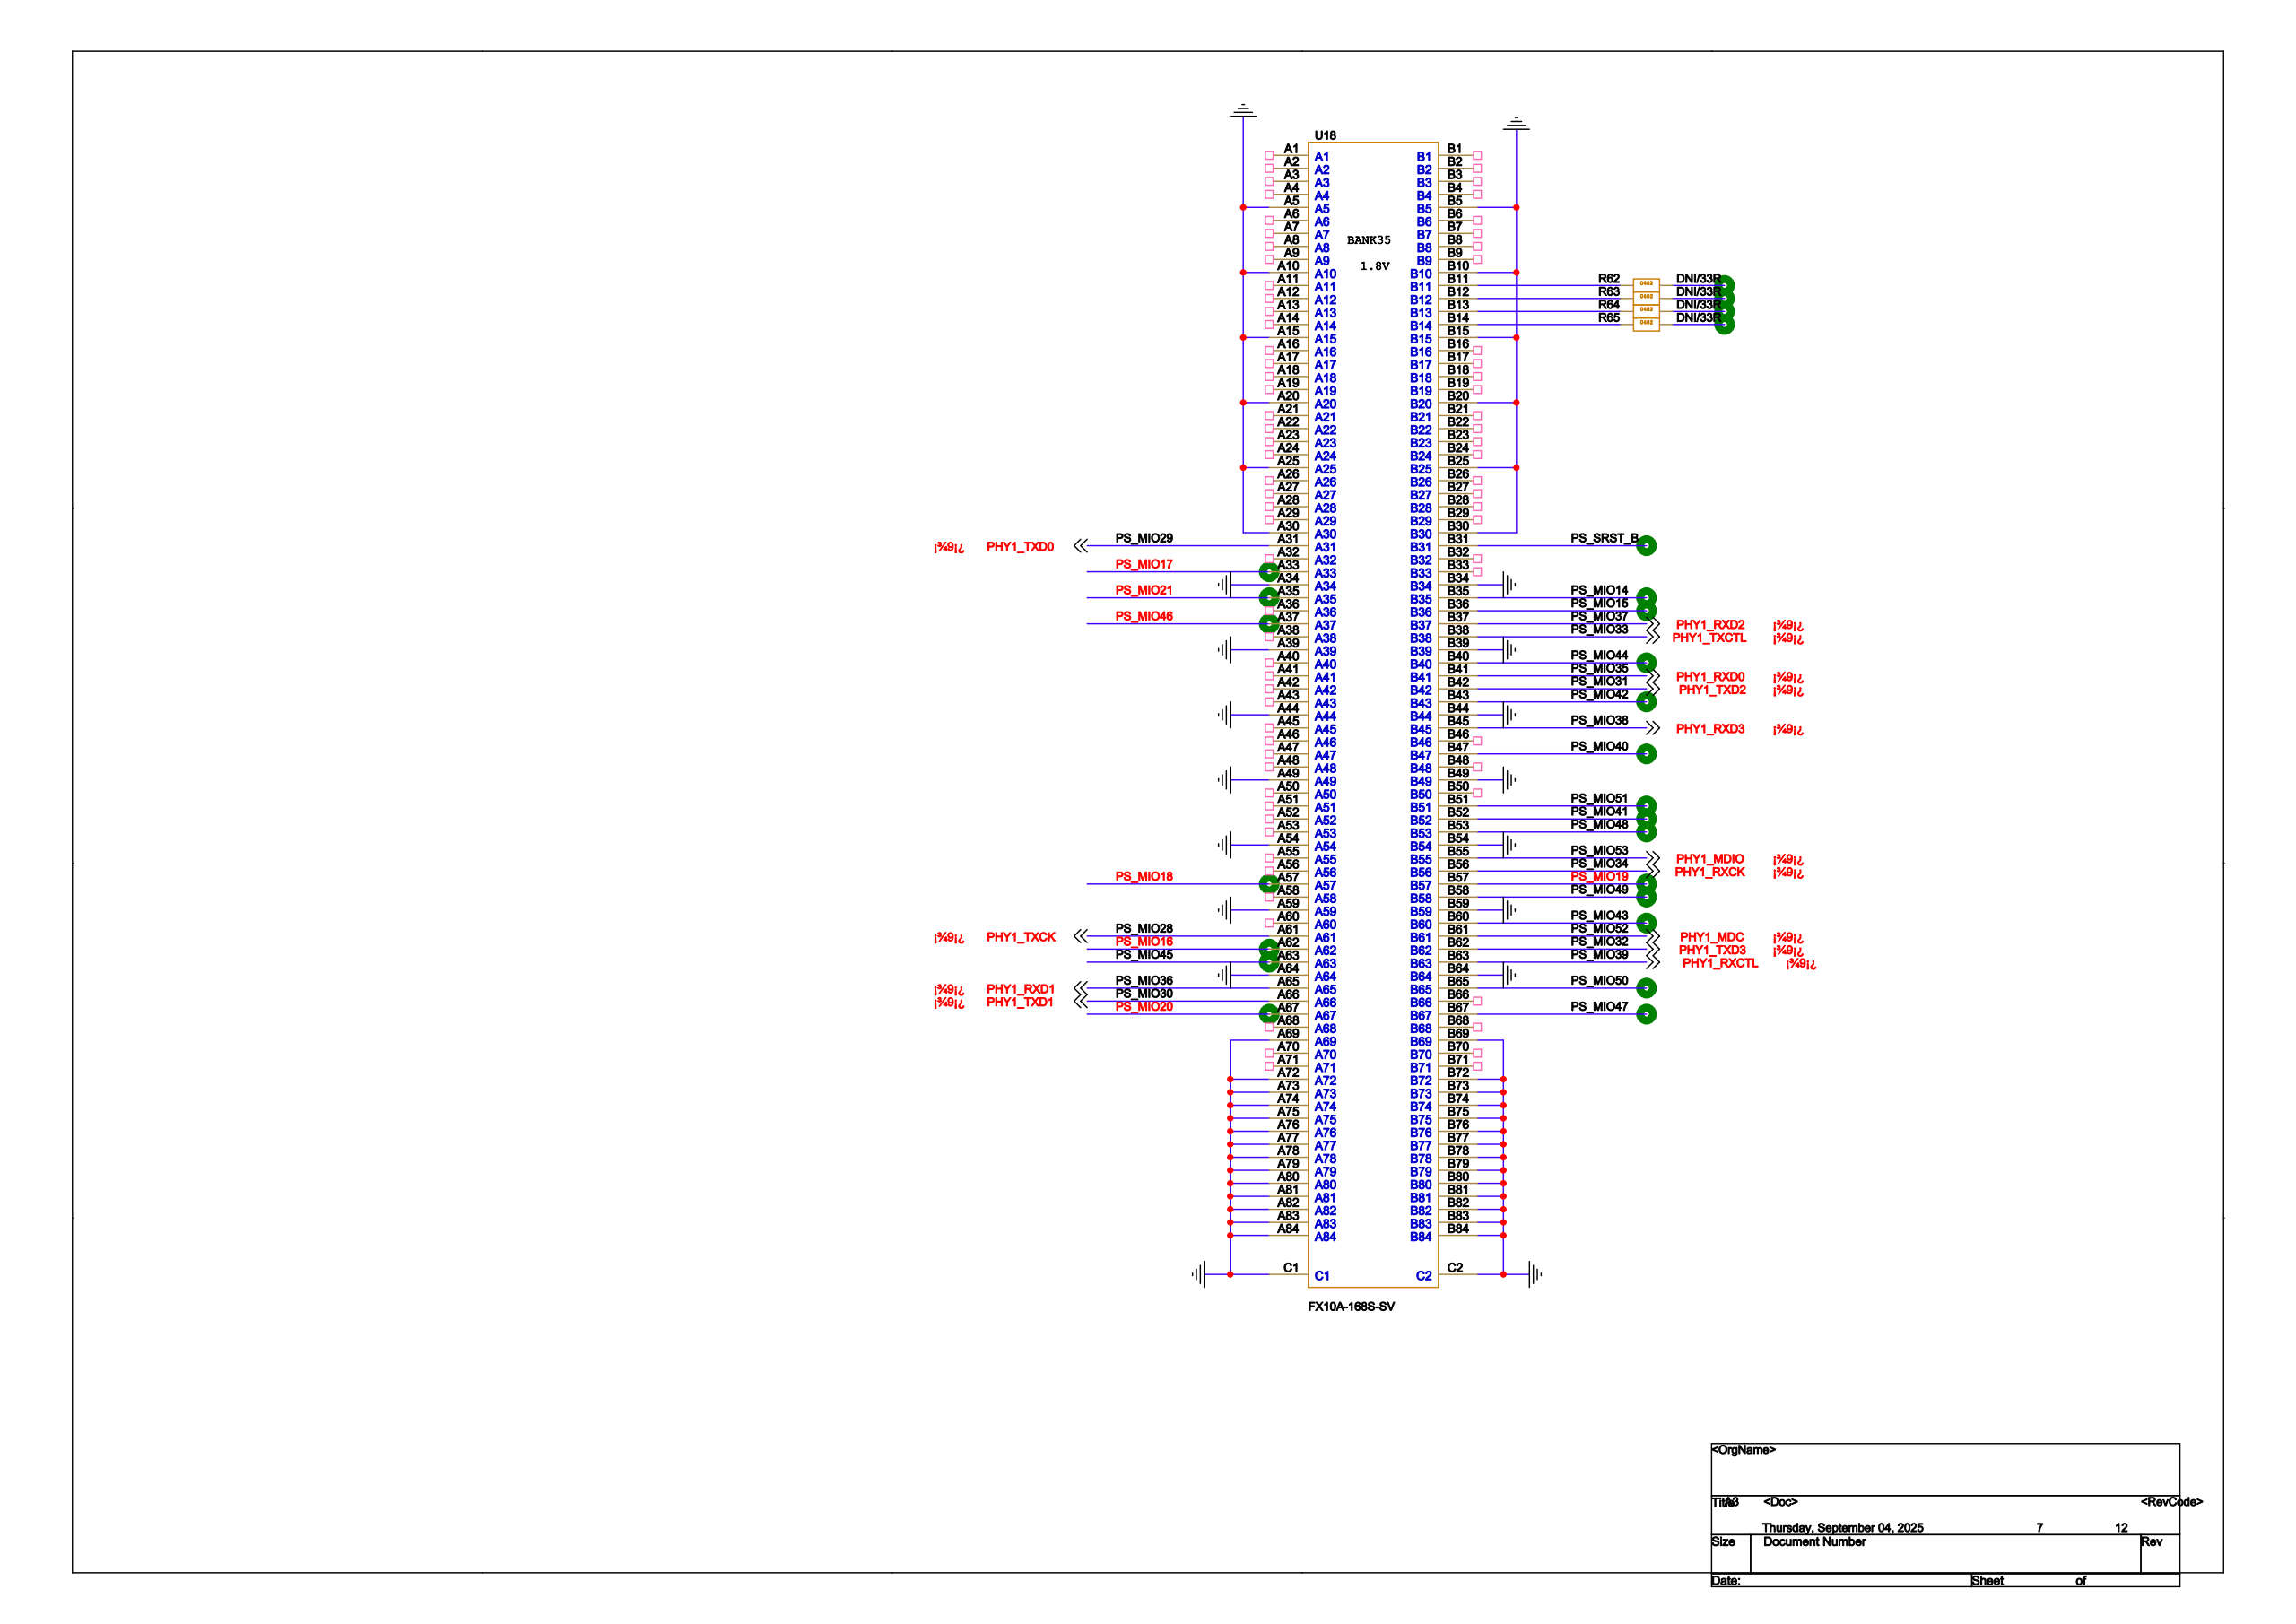Circuit board | Cadence Allegro | 528 parts | 530 nets | one sheet of the schematic
Parts on this sheet (reference | value | footprint):
R62 | DNI/33R | R0402
R63 | DNI/33R | R0402
R64 | DNI/33R | R0402
R65 | DNI/33R | R0402
U18 | FX10A-168S-SV | FX10A-168S-SV
Nets of these parts (net: part-pin ...):
N18098319: R62-1 U18-B11
N18098309: R62-2
N18098323: R63-1 U18-B12
N18098321: R63-2
N18098353: R64-1 U18-B13
N18098343: R64-2
N18098357: R65-1 U18-B14
N18098355: R65-2
PHY1_TXD0: U18-A31
PS_MIO17: U18-A33
PS_MIO21: U18-A35
PS_MIO46: U18-A37
PS_MIO18: U18-A57
PHY1_TXCK: U18-A61
PS_MIO16: U18-A62
PS_MIO45: U18-A63
PHY1_RXD1: U18-A65
PHY1_TXD1: U18-A66
PS_MIO20: U18-A67
PS_SRST_B: U18-B31
PS_MIO14: U18-B35
PS_MIO15: U18-B36
PHY1_RXD2: U18-B37
PHY1_TXCTL: U18-B38
PS_MIO44: U18-B40
PHY1_RXD0: U18-B41
PHY1_TXD2: U18-B42
PS_MIO42: U18-B43
PHY1_RXD3: U18-B45
PS_MIO40: U18-B47
PS_MIO51: U18-B51
PS_MIO41: U18-B52
PS_MIO48: U18-B53
PHY1_MDIO: U18-B55
PHY1_RXCK: U18-B56
PS_MIO19: U18-B57
PS_MIO49: U18-B58
PS_MIO43: U18-B60
PHY1_MDC: U18-B61
PHY1_TXD3: U18-B62
PHY1_RXCTL: U18-B63
PS_MIO50: U18-B65
PS_MIO47: U18-B67